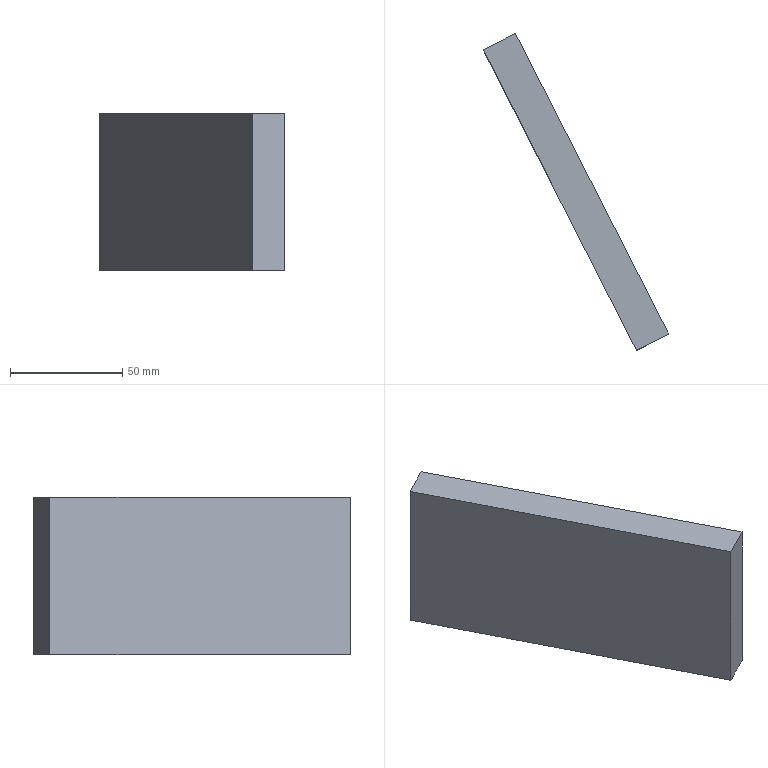Part | NX | features solid 2 | 1 solid | 6 faces | box 82.355 x 140.915 x 70 mm | volume 168000 mm3 | plane 6
STEP:
#1=CARTESIAN_POINT('',(-1754.774,-490.065,250.));
#2=VERTEX_POINT('',#1);
#3=CARTESIAN_POINT('',(-1754.774,-490.065,180.));
#4=VERTEX_POINT('',#3);
#5=CARTESIAN_POINT('',(-1754.774,-490.065,250.));
#6=DIRECTION('',(0.,0.,-1.));
#7=VECTOR('',#6,1000.);
#8=LINE('',#5,#7);
#9=EDGE_CURVE('',#2,#4,#8,.T.);
#10=ORIENTED_EDGE('',*,*,#9,.T.);
#11=CARTESIAN_POINT('',(-1686.676,-623.716,180.));
#12=VERTEX_POINT('',#11);
#13=CARTESIAN_POINT('',(-1686.676,-623.716,180.));
#14=DIRECTION('',(-0.454,0.891,0.));
#15=VECTOR('',#14,1000.);
#16=LINE('',#13,#15);
#17=EDGE_CURVE('',#12,#4,#16,.T.);
#18=ORIENTED_EDGE('',*,*,#17,.F.);
#19=CARTESIAN_POINT('',(-1686.676,-623.716,250.));
#20=VERTEX_POINT('',#19);
#21=CARTESIAN_POINT('',(-1686.676,-623.716,250.));
#22=DIRECTION('',(0.,0.,-1.));
#23=VECTOR('',#22,1000.);
#24=LINE('',#21,#23);
#25=EDGE_CURVE('',#20,#12,#24,.T.);
#26=ORIENTED_EDGE('',*,*,#25,.F.);
#27=CARTESIAN_POINT('',(-1686.676,-623.716,250.));
#28=DIRECTION('',(-0.454,0.891,0.));
#29=VECTOR('',#28,1000.);
#30=LINE('',#27,#29);
#31=EDGE_CURVE('',#20,#2,#30,.T.);
#32=ORIENTED_EDGE('',*,*,#31,.T.);
#33=EDGE_LOOP('',(#10,#18,#26,#32));
#34=FACE_BOUND('',#33,.T.);
#35=CARTESIAN_POINT('',(-1686.676,-623.716,250.));
#36=DIRECTION('',(-0.891,-0.454,0.));
#37=DIRECTION('',(0.,0.,1.));
#38=AXIS2_PLACEMENT_3D('',#35,#36,#37);
#39=PLANE('',#38);
#40=ADVANCED_FACE('',(#34),#39,.T.);
#41=CARTESIAN_POINT('',(-1740.518,-482.801,180.));
#42=VERTEX_POINT('',#41);
#43=CARTESIAN_POINT('',(-1740.518,-482.801,180.));
#44=DIRECTION('',(-0.891,-0.454,0.));
#45=VECTOR('',#44,1000.);
#46=LINE('',#43,#45);
#47=EDGE_CURVE('',#42,#4,#46,.T.);
#48=ORIENTED_EDGE('',*,*,#47,.F.);
#49=CARTESIAN_POINT('',(-1672.42,-616.452,180.));
#50=VERTEX_POINT('',#49);
#51=CARTESIAN_POINT('',(-1672.42,-616.452,180.));
#52=DIRECTION('',(-0.454,0.891,0.));
#53=VECTOR('',#52,1000.);
#54=LINE('',#51,#53);
#55=EDGE_CURVE('',#50,#42,#54,.T.);
#56=ORIENTED_EDGE('',*,*,#55,.F.);
#57=CARTESIAN_POINT('',(-1672.42,-616.452,180.));
#58=DIRECTION('',(-0.891,-0.454,0.));
#59=VECTOR('',#58,1000.);
#60=LINE('',#57,#59);
#61=EDGE_CURVE('',#50,#12,#60,.T.);
#62=ORIENTED_EDGE('',*,*,#61,.T.);
#63=ORIENTED_EDGE('',*,*,#17,.T.);
#64=EDGE_LOOP('',(#48,#56,#62,#63));
#65=FACE_BOUND('',#64,.T.);
#66=CARTESIAN_POINT('',(-1672.42,-616.452,180.));
#67=DIRECTION('',(0.,0.,1.));
#68=DIRECTION('',(0.891,0.454,0.));
#69=AXIS2_PLACEMENT_3D('',#66,#67,#68);
#70=PLANE('',#69);
#71=ADVANCED_FACE('',(#65),#70,.F.);
#72=CARTESIAN_POINT('',(-1740.518,-482.801,250.));
#73=VERTEX_POINT('',#72);
#74=CARTESIAN_POINT('',(-1740.518,-482.801,250.));
#75=DIRECTION('',(0.,0.,-1.));
#76=VECTOR('',#75,1000.);
#77=LINE('',#74,#76);
#78=EDGE_CURVE('',#73,#42,#77,.T.);
#79=ORIENTED_EDGE('',*,*,#78,.F.);
#80=CARTESIAN_POINT('',(-1672.42,-616.452,250.));
#81=VERTEX_POINT('',#80);
#82=CARTESIAN_POINT('',(-1672.42,-616.452,250.));
#83=DIRECTION('',(-0.454,0.891,0.));
#84=VECTOR('',#83,1000.);
#85=LINE('',#82,#84);
#86=EDGE_CURVE('',#81,#73,#85,.T.);
#87=ORIENTED_EDGE('',*,*,#86,.F.);
#88=CARTESIAN_POINT('',(-1672.42,-616.452,250.));
#89=DIRECTION('',(0.,0.,-1.));
#90=VECTOR('',#89,1000.);
#91=LINE('',#88,#90);
#92=EDGE_CURVE('',#81,#50,#91,.T.);
#93=ORIENTED_EDGE('',*,*,#92,.T.);
#94=ORIENTED_EDGE('',*,*,#55,.T.);
#95=EDGE_LOOP('',(#79,#87,#93,#94));
#96=FACE_BOUND('',#95,.T.);
#97=CARTESIAN_POINT('',(-1672.42,-616.452,250.));
#98=DIRECTION('',(-0.891,-0.454,0.));
#99=DIRECTION('',(0.,0.,1.));
#100=AXIS2_PLACEMENT_3D('',#97,#98,#99);
#101=PLANE('',#100);
#102=ADVANCED_FACE('',(#96),#101,.F.);
#103=CARTESIAN_POINT('',(-1740.518,-482.801,250.));
#104=DIRECTION('',(-0.891,-0.454,0.));
#105=VECTOR('',#104,1000.);
#106=LINE('',#103,#105);
#107=EDGE_CURVE('',#73,#2,#106,.T.);
#108=ORIENTED_EDGE('',*,*,#107,.T.);
#109=ORIENTED_EDGE('',*,*,#31,.F.);
#110=CARTESIAN_POINT('',(-1672.42,-616.452,250.));
#111=DIRECTION('',(-0.891,-0.454,0.));
#112=VECTOR('',#111,1000.);
#113=LINE('',#110,#112);
#114=EDGE_CURVE('',#81,#20,#113,.T.);
#115=ORIENTED_EDGE('',*,*,#114,.F.);
#116=ORIENTED_EDGE('',*,*,#86,.T.);
#117=EDGE_LOOP('',(#108,#109,#115,#116));
#118=FACE_BOUND('',#117,.T.);
#119=CARTESIAN_POINT('',(-1672.42,-616.452,250.));
#120=DIRECTION('',(0.,0.,1.));
#121=DIRECTION('',(0.891,0.454,0.));
#122=AXIS2_PLACEMENT_3D('',#119,#120,#121);
#123=PLANE('',#122);
#124=ADVANCED_FACE('',(#118),#123,.T.);
#125=ORIENTED_EDGE('',*,*,#25,.T.);
#126=ORIENTED_EDGE('',*,*,#61,.F.);
#127=ORIENTED_EDGE('',*,*,#92,.F.);
#128=ORIENTED_EDGE('',*,*,#114,.T.);
#129=EDGE_LOOP('',(#125,#126,#127,#128));
#130=FACE_BOUND('',#129,.T.);
#131=CARTESIAN_POINT('',(-1686.676,-623.716,185.));
#132=DIRECTION('',(0.454,-0.891,0.));
#133=DIRECTION('',(0.,0.,1.));
#134=AXIS2_PLACEMENT_3D('',#131,#132,#133);
#135=PLANE('',#134);
#136=ADVANCED_FACE('',(#130),#135,.T.);
#137=ORIENTED_EDGE('',*,*,#9,.F.);
#138=ORIENTED_EDGE('',*,*,#107,.F.);
#139=ORIENTED_EDGE('',*,*,#78,.T.);
#140=ORIENTED_EDGE('',*,*,#47,.T.);
#141=EDGE_LOOP('',(#137,#138,#139,#140));
#142=FACE_BOUND('',#141,.T.);
#143=CARTESIAN_POINT('',(-1754.774,-490.065,185.));
#144=DIRECTION('',(0.454,-0.891,0.));
#145=DIRECTION('',(0.,0.,1.));
#146=AXIS2_PLACEMENT_3D('',#143,#144,#145);
#147=PLANE('',#146);
#148=ADVANCED_FACE('',(#142),#147,.F.);
#149=CLOSED_SHELL('',(#40,#71,#102,#124,#136,#148));
#150=MANIFOLD_SOLID_BREP('',#149);
#151=(LENGTH_UNIT()NAMED_UNIT(*)SI_UNIT(.MILLI.,.METRE.));
#152=UNCERTAINTY_MEASURE_WITH_UNIT(LENGTH_MEASURE(0.00001),#151,'','');
#153=(NAMED_UNIT(*)PLANE_ANGLE_UNIT()SI_UNIT($,.RADIAN.));
#154=(NAMED_UNIT(*)SI_UNIT($,.STERADIAN.)SOLID_ANGLE_UNIT());
#155=(GEOMETRIC_REPRESENTATION_CONTEXT(3)GLOBAL_UNCERTAINTY_ASSIGNED_CONTEXT((#152))GLOBAL_UNIT_ASSIGNED_CONTEXT((#151,#153,#154))REPRESENTATION_CONTEXT('',''));
#156=ADVANCED_BREP_SHAPE_REPRESENTATION('',(#150),#155);